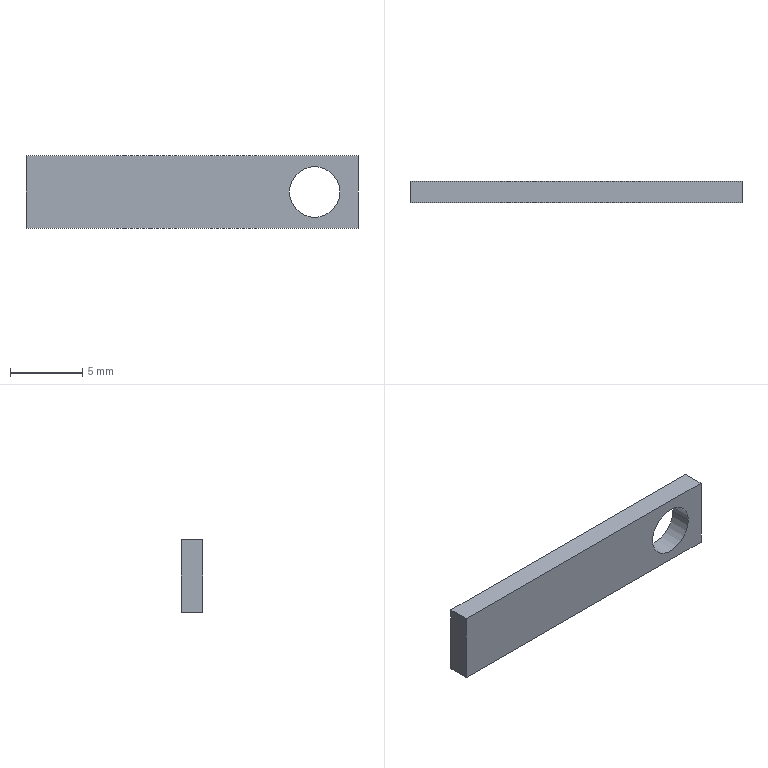Part | NX | 1 solid | 8 faces | box 23 x 1.5 x 5 mm | volume 158.068 mm3 | plane 6 | cylinder 2 | commonest cylinder face diameters 3.5 x2
STEP:
#1=CARTESIAN_POINT('',(-11.5,0.5,0.));
#2=VERTEX_POINT('',#1);
#3=CARTESIAN_POINT('',(-11.5,-1.,0.));
#4=VERTEX_POINT('',#3);
#5=CARTESIAN_POINT('',(-11.5,0.,0.));
#6=DIRECTION('',(0.,-1.,0.));
#7=VECTOR('',#6,1000.);
#8=LINE('',#5,#7);
#9=EDGE_CURVE('',#2,#4,#8,.T.);
#10=ORIENTED_EDGE('',*,*,#9,.F.);
#11=CARTESIAN_POINT('',(11.5,0.5,0.));
#12=VERTEX_POINT('',#11);
#13=CARTESIAN_POINT('',(0.,0.5,0.));
#14=DIRECTION('',(1.,0.,0.));
#15=VECTOR('',#14,1000.);
#16=LINE('',#13,#15);
#17=EDGE_CURVE('',#2,#12,#16,.T.);
#18=ORIENTED_EDGE('',*,*,#17,.T.);
#19=CARTESIAN_POINT('',(11.5,-1.,0.));
#20=VERTEX_POINT('',#19);
#21=CARTESIAN_POINT('',(11.5,0.,0.));
#22=DIRECTION('',(0.,1.,0.));
#23=VECTOR('',#22,1000.);
#24=LINE('',#21,#23);
#25=EDGE_CURVE('',#20,#12,#24,.T.);
#26=ORIENTED_EDGE('',*,*,#25,.F.);
#27=CARTESIAN_POINT('',(0.,-1.,0.));
#28=DIRECTION('',(1.,0.,0.));
#29=VECTOR('',#28,1000.);
#30=LINE('',#27,#29);
#31=EDGE_CURVE('',#4,#20,#30,.T.);
#32=ORIENTED_EDGE('',*,*,#31,.F.);
#33=EDGE_LOOP('',(#10,#18,#26,#32));
#34=FACE_BOUND('',#33,.T.);
#35=CARTESIAN_POINT('',(0.,0.,0.));
#36=DIRECTION('',(0.,0.,1.));
#37=DIRECTION('',(1.,0.,0.));
#38=AXIS2_PLACEMENT_3D('',#35,#36,#37);
#39=PLANE('',#38);
#40=ADVANCED_FACE('',(#34),#39,.F.);
#41=ORIENTED_EDGE('',*,*,#9,.T.);
#42=CARTESIAN_POINT('',(-11.5,-1.,5.));
#43=VERTEX_POINT('',#42);
#44=CARTESIAN_POINT('',(-11.5,-1.,0.));
#45=DIRECTION('',(0.,0.,-1.));
#46=VECTOR('',#45,1000.);
#47=LINE('',#44,#46);
#48=EDGE_CURVE('',#43,#4,#47,.T.);
#49=ORIENTED_EDGE('',*,*,#48,.F.);
#50=CARTESIAN_POINT('',(-11.5,0.5,5.));
#51=VERTEX_POINT('',#50);
#52=CARTESIAN_POINT('',(-11.5,0.,5.));
#53=DIRECTION('',(0.,1.,0.));
#54=VECTOR('',#53,1000.);
#55=LINE('',#52,#54);
#56=EDGE_CURVE('',#43,#51,#55,.T.);
#57=ORIENTED_EDGE('',*,*,#56,.T.);
#58=CARTESIAN_POINT('',(-11.5,0.5,0.));
#59=DIRECTION('',(0.,0.,1.));
#60=VECTOR('',#59,1000.);
#61=LINE('',#58,#60);
#62=EDGE_CURVE('',#2,#51,#61,.T.);
#63=ORIENTED_EDGE('',*,*,#62,.F.);
#64=EDGE_LOOP('',(#41,#49,#57,#63));
#65=FACE_BOUND('',#64,.T.);
#66=CARTESIAN_POINT('',(-11.5,0.5,0.));
#67=DIRECTION('',(-1.,0.,0.));
#68=DIRECTION('',(0.,0.,1.));
#69=AXIS2_PLACEMENT_3D('',#66,#67,#68);
#70=PLANE('',#69);
#71=ADVANCED_FACE('',(#65),#70,.T.);
#72=ORIENTED_EDGE('',*,*,#17,.F.);
#73=ORIENTED_EDGE('',*,*,#62,.T.);
#74=CARTESIAN_POINT('',(11.5,0.5,5.));
#75=VERTEX_POINT('',#74);
#76=CARTESIAN_POINT('',(0.,0.5,5.));
#77=DIRECTION('',(1.,0.,0.));
#78=VECTOR('',#77,1000.);
#79=LINE('',#76,#78);
#80=EDGE_CURVE('',#51,#75,#79,.T.);
#81=ORIENTED_EDGE('',*,*,#80,.T.);
#82=CARTESIAN_POINT('',(11.5,0.5,0.));
#83=DIRECTION('',(0.,0.,-1.));
#84=VECTOR('',#83,1000.);
#85=LINE('',#82,#84);
#86=EDGE_CURVE('',#75,#12,#85,.T.);
#87=ORIENTED_EDGE('',*,*,#86,.T.);
#88=EDGE_LOOP('',(#72,#73,#81,#87));
#89=FACE_BOUND('',#88,.T.);
#90=CARTESIAN_POINT('',(10.25,0.5,2.5));
#91=VERTEX_POINT('',#90);
#92=CARTESIAN_POINT('',(6.75,0.5,2.5));
#93=VERTEX_POINT('',#92);
#94=CARTESIAN_POINT('',(8.5,0.5,2.5));
#95=DIRECTION('',(0.,-1.,0.));
#96=DIRECTION('',(1.,0.,0.));
#97=AXIS2_PLACEMENT_3D('',#94,#95,#96);
#98=CIRCLE('',#97,1.75);
#99=EDGE_CURVE('',#91,#93,#98,.T.);
#100=ORIENTED_EDGE('',*,*,#99,.T.);
#101=CARTESIAN_POINT('',(8.5,0.5,2.5));
#102=DIRECTION('',(0.,-1.,0.));
#103=DIRECTION('',(1.,0.,0.));
#104=AXIS2_PLACEMENT_3D('',#101,#102,#103);
#105=CIRCLE('',#104,1.75);
#106=EDGE_CURVE('',#93,#91,#105,.T.);
#107=ORIENTED_EDGE('',*,*,#106,.T.);
#108=EDGE_LOOP('',(#100,#107));
#109=FACE_BOUND('',#108,.T.);
#110=CARTESIAN_POINT('',(11.5,0.5,0.));
#111=DIRECTION('',(0.,1.,0.));
#112=DIRECTION('',(1.,0.,0.));
#113=AXIS2_PLACEMENT_3D('',#110,#111,#112);
#114=PLANE('',#113);
#115=ADVANCED_FACE('',(#89,#109),#114,.T.);
#116=ORIENTED_EDGE('',*,*,#25,.T.);
#117=ORIENTED_EDGE('',*,*,#86,.F.);
#118=CARTESIAN_POINT('',(11.5,-1.,5.));
#119=VERTEX_POINT('',#118);
#120=CARTESIAN_POINT('',(11.5,0.,5.));
#121=DIRECTION('',(0.,-1.,0.));
#122=VECTOR('',#121,1000.);
#123=LINE('',#120,#122);
#124=EDGE_CURVE('',#75,#119,#123,.T.);
#125=ORIENTED_EDGE('',*,*,#124,.T.);
#126=CARTESIAN_POINT('',(11.5,-1.,0.));
#127=DIRECTION('',(0.,0.,-1.));
#128=VECTOR('',#127,1000.);
#129=LINE('',#126,#128);
#130=EDGE_CURVE('',#119,#20,#129,.T.);
#131=ORIENTED_EDGE('',*,*,#130,.T.);
#132=EDGE_LOOP('',(#116,#117,#125,#131));
#133=FACE_BOUND('',#132,.T.);
#134=CARTESIAN_POINT('',(11.5,-0.5,0.));
#135=DIRECTION('',(1.,0.,0.));
#136=DIRECTION('',(0.,1.,0.));
#137=AXIS2_PLACEMENT_3D('',#134,#135,#136);
#138=PLANE('',#137);
#139=ADVANCED_FACE('',(#133),#138,.T.);
#140=ORIENTED_EDGE('',*,*,#31,.T.);
#141=ORIENTED_EDGE('',*,*,#130,.F.);
#142=CARTESIAN_POINT('',(0.,-1.,5.));
#143=DIRECTION('',(-1.,0.,0.));
#144=VECTOR('',#143,1000.);
#145=LINE('',#142,#144);
#146=EDGE_CURVE('',#119,#43,#145,.T.);
#147=ORIENTED_EDGE('',*,*,#146,.T.);
#148=ORIENTED_EDGE('',*,*,#48,.T.);
#149=EDGE_LOOP('',(#140,#141,#147,#148));
#150=FACE_BOUND('',#149,.T.);
#151=CARTESIAN_POINT('',(10.25,-1.,2.5));
#152=VERTEX_POINT('',#151);
#153=CARTESIAN_POINT('',(6.75,-1.,2.5));
#154=VERTEX_POINT('',#153);
#155=CARTESIAN_POINT('',(8.5,-1.,2.5));
#156=DIRECTION('',(0.,-1.,0.));
#157=DIRECTION('',(1.,0.,0.));
#158=AXIS2_PLACEMENT_3D('',#155,#156,#157);
#159=CIRCLE('',#158,1.75);
#160=EDGE_CURVE('',#152,#154,#159,.T.);
#161=ORIENTED_EDGE('',*,*,#160,.F.);
#162=CARTESIAN_POINT('',(8.5,-1.,2.5));
#163=DIRECTION('',(0.,-1.,0.));
#164=DIRECTION('',(1.,0.,0.));
#165=AXIS2_PLACEMENT_3D('',#162,#163,#164);
#166=CIRCLE('',#165,1.75);
#167=EDGE_CURVE('',#154,#152,#166,.T.);
#168=ORIENTED_EDGE('',*,*,#167,.F.);
#169=EDGE_LOOP('',(#161,#168));
#170=FACE_BOUND('',#169,.T.);
#171=CARTESIAN_POINT('',(-11.5,-1.,0.));
#172=DIRECTION('',(0.,-1.,0.));
#173=DIRECTION('',(0.,0.,-1.));
#174=AXIS2_PLACEMENT_3D('',#171,#172,#173);
#175=PLANE('',#174);
#176=ADVANCED_FACE('',(#150,#170),#175,.T.);
#177=ORIENTED_EDGE('',*,*,#56,.F.);
#178=ORIENTED_EDGE('',*,*,#146,.F.);
#179=ORIENTED_EDGE('',*,*,#124,.F.);
#180=ORIENTED_EDGE('',*,*,#80,.F.);
#181=EDGE_LOOP('',(#177,#178,#179,#180));
#182=FACE_BOUND('',#181,.T.);
#183=CARTESIAN_POINT('',(0.,0.,5.));
#184=DIRECTION('',(0.,0.,1.));
#185=DIRECTION('',(1.,0.,0.));
#186=AXIS2_PLACEMENT_3D('',#183,#184,#185);
#187=PLANE('',#186);
#188=ADVANCED_FACE('',(#182),#187,.T.);
#189=ORIENTED_EDGE('',*,*,#99,.F.);
#190=CARTESIAN_POINT('',(10.25,0.5,2.5));
#191=DIRECTION('',(0.,-1.,0.));
#192=VECTOR('',#191,1000.);
#193=LINE('',#190,#192);
#194=EDGE_CURVE('',#91,#152,#193,.T.);
#195=ORIENTED_EDGE('',*,*,#194,.T.);
#196=ORIENTED_EDGE('',*,*,#160,.T.);
#197=CARTESIAN_POINT('',(6.75,0.5,2.5));
#198=DIRECTION('',(0.,-1.,0.));
#199=VECTOR('',#198,1000.);
#200=LINE('',#197,#199);
#201=EDGE_CURVE('',#93,#154,#200,.T.);
#202=ORIENTED_EDGE('',*,*,#201,.F.);
#203=EDGE_LOOP('',(#189,#195,#196,#202));
#204=FACE_BOUND('',#203,.T.);
#205=CARTESIAN_POINT('',(8.5,0.5,2.5));
#206=DIRECTION('',(0.,-1.,0.));
#207=DIRECTION('',(1.,0.,0.));
#208=AXIS2_PLACEMENT_3D('',#205,#206,#207);
#209=CYLINDRICAL_SURFACE('',#208,1.75);
#210=ADVANCED_FACE('',(#204),#209,.F.);
#211=ORIENTED_EDGE('',*,*,#194,.F.);
#212=ORIENTED_EDGE('',*,*,#106,.F.);
#213=ORIENTED_EDGE('',*,*,#201,.T.);
#214=ORIENTED_EDGE('',*,*,#167,.T.);
#215=EDGE_LOOP('',(#211,#212,#213,#214));
#216=FACE_BOUND('',#215,.T.);
#217=CARTESIAN_POINT('',(8.5,0.5,2.5));
#218=DIRECTION('',(0.,-1.,0.));
#219=DIRECTION('',(1.,0.,0.));
#220=AXIS2_PLACEMENT_3D('',#217,#218,#219);
#221=CYLINDRICAL_SURFACE('',#220,1.75);
#222=ADVANCED_FACE('',(#216),#221,.F.);
#223=CLOSED_SHELL('',(#40,#71,#115,#139,#176,#188,#210,#222));
#224=MANIFOLD_SOLID_BREP('',#223);
#225=(LENGTH_UNIT()NAMED_UNIT(*)SI_UNIT(.MILLI.,.METRE.));
#226=UNCERTAINTY_MEASURE_WITH_UNIT(LENGTH_MEASURE(0.00001),#225,'','');
#227=(NAMED_UNIT(*)PLANE_ANGLE_UNIT()SI_UNIT($,.RADIAN.));
#228=(NAMED_UNIT(*)SI_UNIT($,.STERADIAN.)SOLID_ANGLE_UNIT());
#229=(GEOMETRIC_REPRESENTATION_CONTEXT(3)GLOBAL_UNCERTAINTY_ASSIGNED_CONTEXT((#226))GLOBAL_UNIT_ASSIGNED_CONTEXT((#225,#227,#228))REPRESENTATION_CONTEXT('',''));
#230=ADVANCED_BREP_SHAPE_REPRESENTATION('',(#224),#229);